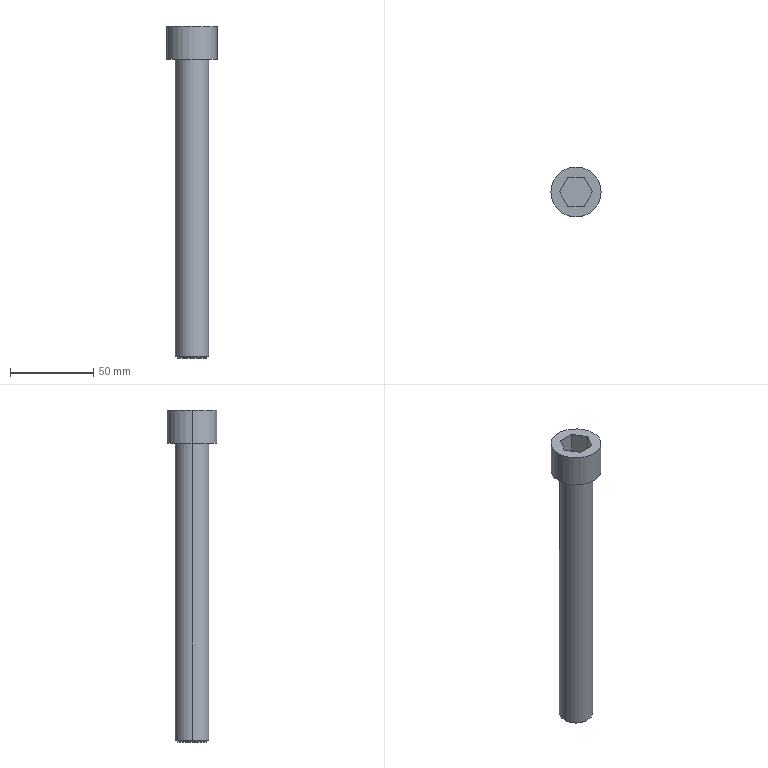Part | Creo | 1 solid | 16 faces | box 30 x 30 x 199 mm | volume 67037 mm3 | plane 10 | cylinder 4 | cone 2 | commonest cylinder face diameters 20 x2 30 x2
STEP:
#1=CARTESIAN_POINT('',(0.,0.,0.));
#2=DIRECTION('',(0.,0.,1.));
#3=DIRECTION('',(1.,0.,0.));
#4=AXIS2_PLACEMENT_3D('',#1,#2,#3);
#5=CARTESIAN_POINT('',(-295.899,-189.627,172.573));
#6=VERTEX_POINT('',#5);
#7=CARTESIAN_POINT('',(-275.899,-189.627,172.573));
#8=VERTEX_POINT('',#7);
#9=CARTESIAN_POINT('',(-285.899,-189.627,172.573));
#10=DIRECTION('',(0.,0.,-1.));
#11=DIRECTION('',(-1.,0.,0.));
#12=AXIS2_PLACEMENT_3D('',#9,#10,#11);
#13=CIRCLE('',#12,10.);
#14=EDGE_CURVE('',#6,#8,#13,.T.);
#15=ORIENTED_EDGE('',*,*,#14,.T.);
#16=CARTESIAN_POINT('',(-275.899,-189.627,350.559));
#17=VERTEX_POINT('',#16);
#18=CARTESIAN_POINT('',(-275.899,-189.627,350.559));
#19=DIRECTION('',(0.,0.,-1.));
#20=VECTOR('',#19,177.985);
#21=LINE('',#18,#20);
#22=EDGE_CURVE('',#17,#8,#21,.T.);
#23=ORIENTED_EDGE('',*,*,#22,.F.);
#24=CARTESIAN_POINT('',(-295.899,-189.627,350.559));
#25=VERTEX_POINT('',#24);
#26=CARTESIAN_POINT('',(-285.899,-189.627,350.559));
#27=DIRECTION('',(0.,0.,1.));
#28=DIRECTION('',(1.,0.,0.));
#29=AXIS2_PLACEMENT_3D('',#26,#27,#28);
#30=CIRCLE('',#29,10.);
#31=EDGE_CURVE('',#17,#25,#30,.T.);
#32=ORIENTED_EDGE('',*,*,#31,.T.);
#33=CARTESIAN_POINT('',(-295.899,-189.627,350.559));
#34=DIRECTION('',(0.,0.,-1.));
#35=VECTOR('',#34,177.985);
#36=LINE('',#33,#35);
#37=EDGE_CURVE('',#25,#6,#36,.T.);
#38=ORIENTED_EDGE('',*,*,#37,.T.);
#39=EDGE_LOOP('',(#15,#23,#32,#38));
#40=FACE_OUTER_BOUND('',#39,.F.);
#41=CARTESIAN_POINT('',(-285.899,-189.627,350.559));
#42=DIRECTION('',(0.,0.,-1.));
#43=DIRECTION('',(-1.,0.,0.));
#44=AXIS2_PLACEMENT_3D('',#41,#42,#43);
#45=CYLINDRICAL_SURFACE('',#44,10.);
#46=ADVANCED_FACE('',(#40),#45,.T.);
#47=CARTESIAN_POINT('',(-294.884,-189.627,171.559));
#48=VERTEX_POINT('',#47);
#49=CARTESIAN_POINT('',(-276.914,-189.627,171.559));
#50=VERTEX_POINT('',#49);
#51=CARTESIAN_POINT('',(-285.899,-189.627,171.559));
#52=DIRECTION('',(0.,0.,-1.));
#53=DIRECTION('',(-1.,0.,0.));
#54=AXIS2_PLACEMENT_3D('',#51,#52,#53);
#55=CIRCLE('',#54,8.985);
#56=EDGE_CURVE('',#48,#50,#55,.T.);
#57=ORIENTED_EDGE('',*,*,#56,.T.);
#58=CARTESIAN_POINT('',(-276.914,-189.627,171.559));
#59=DIRECTION('',(0.7071,0.,0.7071));
#60=VECTOR('',#59,1.435);
#61=LINE('',#58,#60);
#62=EDGE_CURVE('',#50,#8,#61,.T.);
#63=ORIENTED_EDGE('',*,*,#62,.T.);
#64=ORIENTED_EDGE('',*,*,#14,.F.);
#65=CARTESIAN_POINT('',(-294.884,-189.627,171.559));
#66=DIRECTION('',(-0.7071,0.,0.7071));
#67=VECTOR('',#66,1.435);
#68=LINE('',#65,#67);
#69=EDGE_CURVE('',#48,#6,#68,.T.);
#70=ORIENTED_EDGE('',*,*,#69,.F.);
#71=EDGE_LOOP('',(#57,#63,#64,#70));
#72=FACE_OUTER_BOUND('',#71,.F.);
#73=CARTESIAN_POINT('',(-285.899,-189.627,172.066));
#74=DIRECTION('',(0.,0.,1.));
#75=DIRECTION('',(1.,0.,0.));
#76=AXIS2_PLACEMENT_3D('',#73,#74,#75);
#77=CONICAL_SURFACE('',#76,9.493,45.);
#78=ADVANCED_FACE('',(#72),#77,.T.);
#79=CARTESIAN_POINT('',(-285.899,-189.627,171.559));
#80=DIRECTION('',(0.,0.,-1.));
#81=DIRECTION('',(1.,0.,0.));
#82=AXIS2_PLACEMENT_3D('',#79,#80,#81);
#83=CIRCLE('',#82,8.985);
#84=EDGE_CURVE('',#50,#48,#83,.T.);
#85=ORIENTED_EDGE('',*,*,#84,.F.);
#86=ORIENTED_EDGE('',*,*,#56,.F.);
#87=EDGE_LOOP('',(#85,#86));
#88=FACE_OUTER_BOUND('',#87,.F.);
#89=CARTESIAN_POINT('',(-285.899,-189.627,171.559));
#90=DIRECTION('',(0.,0.,1.));
#91=DIRECTION('',(1.,0.,0.));
#92=AXIS2_PLACEMENT_3D('',#89,#90,#91);
#93=PLANE('',#92);
#94=ADVANCED_FACE('',(#88),#93,.F.);
#95=ORIENTED_EDGE('',*,*,#84,.T.);
#96=ORIENTED_EDGE('',*,*,#69,.T.);
#97=CARTESIAN_POINT('',(-285.899,-189.627,172.573));
#98=DIRECTION('',(0.,0.,-1.));
#99=DIRECTION('',(1.,0.,0.));
#100=AXIS2_PLACEMENT_3D('',#97,#98,#99);
#101=CIRCLE('',#100,10.);
#102=EDGE_CURVE('',#8,#6,#101,.T.);
#103=ORIENTED_EDGE('',*,*,#102,.F.);
#104=ORIENTED_EDGE('',*,*,#62,.F.);
#105=EDGE_LOOP('',(#95,#96,#103,#104));
#106=FACE_OUTER_BOUND('',#105,.F.);
#107=CARTESIAN_POINT('',(-285.899,-189.627,172.066));
#108=DIRECTION('',(0.,0.,1.));
#109=DIRECTION('',(1.,0.,0.));
#110=AXIS2_PLACEMENT_3D('',#107,#108,#109);
#111=CONICAL_SURFACE('',#110,9.493,45.);
#112=ADVANCED_FACE('',(#106),#111,.T.);
#113=ORIENTED_EDGE('',*,*,#102,.T.);
#114=ORIENTED_EDGE('',*,*,#37,.F.);
#115=CARTESIAN_POINT('',(-285.899,-189.627,350.559));
#116=DIRECTION('',(0.,0.,1.));
#117=DIRECTION('',(-1.,0.,0.));
#118=AXIS2_PLACEMENT_3D('',#115,#116,#117);
#119=CIRCLE('',#118,10.);
#120=EDGE_CURVE('',#25,#17,#119,.T.);
#121=ORIENTED_EDGE('',*,*,#120,.T.);
#122=ORIENTED_EDGE('',*,*,#22,.T.);
#123=EDGE_LOOP('',(#113,#114,#121,#122));
#124=FACE_OUTER_BOUND('',#123,.F.);
#125=CARTESIAN_POINT('',(-285.899,-189.627,350.559));
#126=DIRECTION('',(0.,0.,-1.));
#127=DIRECTION('',(-1.,0.,0.));
#128=AXIS2_PLACEMENT_3D('',#125,#126,#127);
#129=CYLINDRICAL_SURFACE('',#128,10.);
#130=ADVANCED_FACE('',(#124),#129,.T.);
#131=CARTESIAN_POINT('',(-270.899,-189.627,350.559));
#132=VERTEX_POINT('',#131);
#133=CARTESIAN_POINT('',(-300.899,-189.627,350.559));
#134=VERTEX_POINT('',#133);
#135=CARTESIAN_POINT('',(-285.899,-189.627,350.559));
#136=DIRECTION('',(0.,0.,-1.));
#137=DIRECTION('',(1.,0.,0.));
#138=AXIS2_PLACEMENT_3D('',#135,#136,#137);
#139=CIRCLE('',#138,15.);
#140=EDGE_CURVE('',#132,#134,#139,.T.);
#141=ORIENTED_EDGE('',*,*,#140,.F.);
#142=CARTESIAN_POINT('',(-285.899,-189.627,350.559));
#143=DIRECTION('',(0.,0.,-1.));
#144=DIRECTION('',(-1.,0.,0.));
#145=AXIS2_PLACEMENT_3D('',#142,#143,#144);
#146=CIRCLE('',#145,15.);
#147=EDGE_CURVE('',#134,#132,#146,.T.);
#148=ORIENTED_EDGE('',*,*,#147,.F.);
#149=EDGE_LOOP('',(#141,#148));
#150=FACE_OUTER_BOUND('',#149,.F.);
#151=ORIENTED_EDGE('',*,*,#31,.F.);
#152=ORIENTED_EDGE('',*,*,#120,.F.);
#153=EDGE_LOOP('',(#151,#152));
#154=FACE_BOUND('',#153,.F.);
#155=CARTESIAN_POINT('',(-285.899,-189.627,350.559));
#156=DIRECTION('',(0.,0.,-1.));
#157=DIRECTION('',(-1.,0.,0.));
#158=AXIS2_PLACEMENT_3D('',#155,#156,#157);
#159=PLANE('',#158);
#160=ADVANCED_FACE('',(#150,#154),#159,.T.);
#161=CARTESIAN_POINT('',(-300.899,-189.627,370.559));
#162=VERTEX_POINT('',#161);
#163=CARTESIAN_POINT('',(-270.899,-189.627,370.559));
#164=VERTEX_POINT('',#163);
#165=CARTESIAN_POINT('',(-285.899,-189.627,370.559));
#166=DIRECTION('',(0.,0.,1.));
#167=DIRECTION('',(-1.,0.,0.));
#168=AXIS2_PLACEMENT_3D('',#165,#166,#167);
#169=CIRCLE('',#168,15.);
#170=EDGE_CURVE('',#162,#164,#169,.T.);
#171=ORIENTED_EDGE('',*,*,#170,.T.);
#172=CARTESIAN_POINT('',(-270.899,-189.627,350.559));
#173=DIRECTION('',(0.,0.,1.));
#174=VECTOR('',#173,20.);
#175=LINE('',#172,#174);
#176=EDGE_CURVE('',#132,#164,#175,.T.);
#177=ORIENTED_EDGE('',*,*,#176,.F.);
#178=ORIENTED_EDGE('',*,*,#140,.T.);
#179=CARTESIAN_POINT('',(-300.899,-189.627,350.559));
#180=DIRECTION('',(0.,0.,1.));
#181=VECTOR('',#180,20.);
#182=LINE('',#179,#181);
#183=EDGE_CURVE('',#134,#162,#182,.T.);
#184=ORIENTED_EDGE('',*,*,#183,.T.);
#185=EDGE_LOOP('',(#171,#177,#178,#184));
#186=FACE_OUTER_BOUND('',#185,.F.);
#187=CARTESIAN_POINT('',(-285.899,-189.627,350.559));
#188=DIRECTION('',(0.,0.,1.));
#189=DIRECTION('',(1.,0.,0.));
#190=AXIS2_PLACEMENT_3D('',#187,#188,#189);
#191=CYLINDRICAL_SURFACE('',#190,15.);
#192=ADVANCED_FACE('',(#186),#191,.T.);
#193=CARTESIAN_POINT('',(-285.899,-189.627,370.559));
#194=DIRECTION('',(0.,0.,1.));
#195=DIRECTION('',(1.,0.,0.));
#196=AXIS2_PLACEMENT_3D('',#193,#194,#195);
#197=CIRCLE('',#196,15.);
#198=EDGE_CURVE('',#164,#162,#197,.T.);
#199=ORIENTED_EDGE('',*,*,#198,.F.);
#200=ORIENTED_EDGE('',*,*,#170,.F.);
#201=EDGE_LOOP('',(#199,#200));
#202=FACE_OUTER_BOUND('',#201,.F.);
#203=CARTESIAN_POINT('',(-280.992,-198.127,370.559));
#204=VERTEX_POINT('',#203);
#205=CARTESIAN_POINT('',(-290.807,-198.127,370.559));
#206=VERTEX_POINT('',#205);
#207=CARTESIAN_POINT('',(-280.992,-198.127,370.559));
#208=DIRECTION('',(-1.,0.,0.));
#209=VECTOR('',#208,9.815);
#210=LINE('',#207,#209);
#211=EDGE_CURVE('',#204,#206,#210,.T.);
#212=ORIENTED_EDGE('',*,*,#211,.F.);
#213=CARTESIAN_POINT('',(-276.084,-189.627,370.559));
#214=VERTEX_POINT('',#213);
#215=CARTESIAN_POINT('',(-276.084,-189.627,370.559));
#216=DIRECTION('',(-0.5,-0.866,0.));
#217=VECTOR('',#216,9.815);
#218=LINE('',#215,#217);
#219=EDGE_CURVE('',#214,#204,#218,.T.);
#220=ORIENTED_EDGE('',*,*,#219,.F.);
#221=CARTESIAN_POINT('',(-280.992,-181.127,370.559));
#222=VERTEX_POINT('',#221);
#223=CARTESIAN_POINT('',(-280.992,-181.127,370.559));
#224=DIRECTION('',(0.5,-0.866,0.));
#225=VECTOR('',#224,9.815);
#226=LINE('',#223,#225);
#227=EDGE_CURVE('',#222,#214,#226,.T.);
#228=ORIENTED_EDGE('',*,*,#227,.F.);
#229=CARTESIAN_POINT('',(-290.807,-181.127,370.559));
#230=VERTEX_POINT('',#229);
#231=CARTESIAN_POINT('',(-290.807,-181.127,370.559));
#232=DIRECTION('',(1.,0.,0.));
#233=VECTOR('',#232,9.815);
#234=LINE('',#231,#233);
#235=EDGE_CURVE('',#230,#222,#234,.T.);
#236=ORIENTED_EDGE('',*,*,#235,.F.);
#237=CARTESIAN_POINT('',(-295.714,-189.627,370.559));
#238=VERTEX_POINT('',#237);
#239=CARTESIAN_POINT('',(-295.714,-189.627,370.559));
#240=DIRECTION('',(0.5,0.866,0.));
#241=VECTOR('',#240,9.815);
#242=LINE('',#239,#241);
#243=EDGE_CURVE('',#238,#230,#242,.T.);
#244=ORIENTED_EDGE('',*,*,#243,.F.);
#245=CARTESIAN_POINT('',(-290.807,-198.127,370.559));
#246=DIRECTION('',(-0.5,0.866,0.));
#247=VECTOR('',#246,9.815);
#248=LINE('',#245,#247);
#249=EDGE_CURVE('',#206,#238,#248,.T.);
#250=ORIENTED_EDGE('',*,*,#249,.F.);
#251=EDGE_LOOP('',(#212,#220,#228,#236,#244,#250));
#252=FACE_BOUND('',#251,.F.);
#253=CARTESIAN_POINT('',(-285.899,-189.627,370.559));
#254=DIRECTION('',(0.,0.,1.));
#255=DIRECTION('',(1.,0.,0.));
#256=AXIS2_PLACEMENT_3D('',#253,#254,#255);
#257=PLANE('',#256);
#258=ADVANCED_FACE('',(#202,#252),#257,.T.);
#259=ORIENTED_EDGE('',*,*,#211,.T.);
#260=CARTESIAN_POINT('',(-290.807,-198.127,357.359));
#261=VERTEX_POINT('',#260);
#262=CARTESIAN_POINT('',(-290.807,-198.127,370.559));
#263=DIRECTION('',(0.,0.,-1.));
#264=VECTOR('',#263,13.2);
#265=LINE('',#262,#264);
#266=EDGE_CURVE('',#206,#261,#265,.T.);
#267=ORIENTED_EDGE('',*,*,#266,.T.);
#268=CARTESIAN_POINT('',(-280.992,-198.127,357.359));
#269=VERTEX_POINT('',#268);
#270=CARTESIAN_POINT('',(-280.992,-198.127,357.359));
#271=DIRECTION('',(-1.,0.,0.));
#272=VECTOR('',#271,9.815);
#273=LINE('',#270,#272);
#274=EDGE_CURVE('',#269,#261,#273,.T.);
#275=ORIENTED_EDGE('',*,*,#274,.F.);
#276=CARTESIAN_POINT('',(-280.992,-198.127,370.559));
#277=DIRECTION('',(0.,0.,-1.));
#278=VECTOR('',#277,13.2);
#279=LINE('',#276,#278);
#280=EDGE_CURVE('',#204,#269,#279,.T.);
#281=ORIENTED_EDGE('',*,*,#280,.F.);
#282=EDGE_LOOP('',(#259,#267,#275,#281));
#283=FACE_OUTER_BOUND('',#282,.F.);
#284=CARTESIAN_POINT('',(-290.807,-198.127,357.359));
#285=DIRECTION('',(0.,-1.,0.));
#286=DIRECTION('',(0.,0.,-1.));
#287=AXIS2_PLACEMENT_3D('',#284,#285,#286);
#288=PLANE('',#287);
#289=ADVANCED_FACE('',(#283),#288,.F.);
#290=ORIENTED_EDGE('',*,*,#249,.T.);
#291=CARTESIAN_POINT('',(-295.714,-189.627,357.359));
#292=VERTEX_POINT('',#291);
#293=CARTESIAN_POINT('',(-295.714,-189.627,370.559));
#294=DIRECTION('',(0.,0.,-1.));
#295=VECTOR('',#294,13.2);
#296=LINE('',#293,#295);
#297=EDGE_CURVE('',#238,#292,#296,.T.);
#298=ORIENTED_EDGE('',*,*,#297,.T.);
#299=CARTESIAN_POINT('',(-295.714,-189.627,357.359));
#300=DIRECTION('',(0.5,-0.866,0.));
#301=VECTOR('',#300,9.815);
#302=LINE('',#299,#301);
#303=EDGE_CURVE('',#292,#261,#302,.T.);
#304=ORIENTED_EDGE('',*,*,#303,.T.);
#305=ORIENTED_EDGE('',*,*,#266,.F.);
#306=EDGE_LOOP('',(#290,#298,#304,#305));
#307=FACE_OUTER_BOUND('',#306,.F.);
#308=CARTESIAN_POINT('',(-295.714,-189.627,357.359));
#309=DIRECTION('',(-0.866,-0.5,0.));
#310=DIRECTION('',(0.5,-0.866,0.));
#311=AXIS2_PLACEMENT_3D('',#308,#309,#310);
#312=PLANE('',#311);
#313=ADVANCED_FACE('',(#307),#312,.F.);
#314=ORIENTED_EDGE('',*,*,#243,.T.);
#315=CARTESIAN_POINT('',(-290.807,-181.127,357.359));
#316=VERTEX_POINT('',#315);
#317=CARTESIAN_POINT('',(-290.807,-181.127,370.559));
#318=DIRECTION('',(0.,0.,-1.));
#319=VECTOR('',#318,13.2);
#320=LINE('',#317,#319);
#321=EDGE_CURVE('',#230,#316,#320,.T.);
#322=ORIENTED_EDGE('',*,*,#321,.T.);
#323=CARTESIAN_POINT('',(-290.807,-181.127,357.359));
#324=DIRECTION('',(-0.5,-0.866,0.));
#325=VECTOR('',#324,9.815);
#326=LINE('',#323,#325);
#327=EDGE_CURVE('',#316,#292,#326,.T.);
#328=ORIENTED_EDGE('',*,*,#327,.T.);
#329=ORIENTED_EDGE('',*,*,#297,.F.);
#330=EDGE_LOOP('',(#314,#322,#328,#329));
#331=FACE_OUTER_BOUND('',#330,.F.);
#332=CARTESIAN_POINT('',(-290.807,-181.127,357.359));
#333=DIRECTION('',(-0.866,0.5,0.));
#334=DIRECTION('',(-0.5,-0.866,0.));
#335=AXIS2_PLACEMENT_3D('',#332,#333,#334);
#336=PLANE('',#335);
#337=ADVANCED_FACE('',(#331),#336,.F.);
#338=ORIENTED_EDGE('',*,*,#235,.T.);
#339=CARTESIAN_POINT('',(-280.992,-181.127,357.359));
#340=VERTEX_POINT('',#339);
#341=CARTESIAN_POINT('',(-280.992,-181.127,370.559));
#342=DIRECTION('',(0.,0.,-1.));
#343=VECTOR('',#342,13.2);
#344=LINE('',#341,#343);
#345=EDGE_CURVE('',#222,#340,#344,.T.);
#346=ORIENTED_EDGE('',*,*,#345,.T.);
#347=CARTESIAN_POINT('',(-290.807,-181.127,357.359));
#348=DIRECTION('',(1.,0.,0.));
#349=VECTOR('',#348,9.815);
#350=LINE('',#347,#349);
#351=EDGE_CURVE('',#316,#340,#350,.T.);
#352=ORIENTED_EDGE('',*,*,#351,.F.);
#353=ORIENTED_EDGE('',*,*,#321,.F.);
#354=EDGE_LOOP('',(#338,#346,#352,#353));
#355=FACE_OUTER_BOUND('',#354,.F.);
#356=CARTESIAN_POINT('',(-280.992,-181.127,357.359));
#357=DIRECTION('',(0.,1.,0.));
#358=DIRECTION('',(0.,0.,1.));
#359=AXIS2_PLACEMENT_3D('',#356,#357,#358);
#360=PLANE('',#359);
#361=ADVANCED_FACE('',(#355),#360,.F.);
#362=ORIENTED_EDGE('',*,*,#227,.T.);
#363=CARTESIAN_POINT('',(-276.084,-189.627,357.359));
#364=VERTEX_POINT('',#363);
#365=CARTESIAN_POINT('',(-276.084,-189.627,370.559));
#366=DIRECTION('',(0.,0.,-1.));
#367=VECTOR('',#366,13.2);
#368=LINE('',#365,#367);
#369=EDGE_CURVE('',#214,#364,#368,.T.);
#370=ORIENTED_EDGE('',*,*,#369,.T.);
#371=CARTESIAN_POINT('',(-276.084,-189.627,357.359));
#372=DIRECTION('',(-0.5,0.866,0.));
#373=VECTOR('',#372,9.815);
#374=LINE('',#371,#373);
#375=EDGE_CURVE('',#364,#340,#374,.T.);
#376=ORIENTED_EDGE('',*,*,#375,.T.);
#377=ORIENTED_EDGE('',*,*,#345,.F.);
#378=EDGE_LOOP('',(#362,#370,#376,#377));
#379=FACE_OUTER_BOUND('',#378,.F.);
#380=CARTESIAN_POINT('',(-276.084,-189.627,357.359));
#381=DIRECTION('',(0.866,0.5,0.));
#382=DIRECTION('',(-0.5,0.866,0.));
#383=AXIS2_PLACEMENT_3D('',#380,#381,#382);
#384=PLANE('',#383);
#385=ADVANCED_FACE('',(#379),#384,.F.);
#386=ORIENTED_EDGE('',*,*,#219,.T.);
#387=ORIENTED_EDGE('',*,*,#280,.T.);
#388=CARTESIAN_POINT('',(-280.992,-198.127,357.359));
#389=DIRECTION('',(0.5,0.866,0.));
#390=VECTOR('',#389,9.815);
#391=LINE('',#388,#390);
#392=EDGE_CURVE('',#269,#364,#391,.T.);
#393=ORIENTED_EDGE('',*,*,#392,.T.);
#394=ORIENTED_EDGE('',*,*,#369,.F.);
#395=EDGE_LOOP('',(#386,#387,#393,#394));
#396=FACE_OUTER_BOUND('',#395,.F.);
#397=CARTESIAN_POINT('',(-280.992,-198.127,357.359));
#398=DIRECTION('',(0.866,-0.5,0.));
#399=DIRECTION('',(0.5,0.866,0.));
#400=AXIS2_PLACEMENT_3D('',#397,#398,#399);
#401=PLANE('',#400);
#402=ADVANCED_FACE('',(#396),#401,.F.);
#403=ORIENTED_EDGE('',*,*,#274,.T.);
#404=ORIENTED_EDGE('',*,*,#303,.F.);
#405=ORIENTED_EDGE('',*,*,#327,.F.);
#406=ORIENTED_EDGE('',*,*,#351,.T.);
#407=ORIENTED_EDGE('',*,*,#375,.F.);
#408=ORIENTED_EDGE('',*,*,#392,.F.);
#409=EDGE_LOOP('',(#403,#404,#405,#406,#407,#408));
#410=FACE_OUTER_BOUND('',#409,.F.);
#411=CARTESIAN_POINT('',(-280.992,-198.127,357.359));
#412=DIRECTION('',(0.,0.,1.));
#413=DIRECTION('',(1.,0.,0.));
#414=AXIS2_PLACEMENT_3D('',#411,#412,#413);
#415=PLANE('',#414);
#416=ADVANCED_FACE('',(#410),#415,.T.);
#417=ORIENTED_EDGE('',*,*,#198,.T.);
#418=ORIENTED_EDGE('',*,*,#183,.F.);
#419=ORIENTED_EDGE('',*,*,#147,.T.);
#420=ORIENTED_EDGE('',*,*,#176,.T.);
#421=EDGE_LOOP('',(#417,#418,#419,#420));
#422=FACE_OUTER_BOUND('',#421,.F.);
#423=CARTESIAN_POINT('',(-285.899,-189.627,350.559));
#424=DIRECTION('',(0.,0.,1.));
#425=DIRECTION('',(1.,0.,0.));
#426=AXIS2_PLACEMENT_3D('',#423,#424,#425);
#427=CYLINDRICAL_SURFACE('',#426,15.);
#428=ADVANCED_FACE('',(#422),#427,.T.);
#429=CLOSED_SHELL('',(#46,#78,#94,#112,#130,#160,#192,#258,#289,#313,#337,#361,#385,#402,#416,#428));
#430=MANIFOLD_SOLID_BREP('',#429);
#431=(LENGTH_UNIT()NAMED_UNIT(*)SI_UNIT(.MILLI.,.METRE.));
#432=UNCERTAINTY_MEASURE_WITH_UNIT(LENGTH_MEASURE(0.02035),#431,'','');
#433=(NAMED_UNIT(*)PLANE_ANGLE_UNIT()SI_UNIT($,.RADIAN.));
#434=PLANE_ANGLE_MEASURE_WITH_UNIT(PLANE_ANGLE_MEASURE(0.01745),#433);
#435=(CONVERSION_BASED_UNIT('DEGREE',#434)NAMED_UNIT(*)PLANE_ANGLE_UNIT());
#436=(NAMED_UNIT(*)SI_UNIT($,.STERADIAN.)SOLID_ANGLE_UNIT());
#437=(GEOMETRIC_REPRESENTATION_CONTEXT(3)GLOBAL_UNCERTAINTY_ASSIGNED_CONTEXT((#432))GLOBAL_UNIT_ASSIGNED_CONTEXT((#431,#435,#436))REPRESENTATION_CONTEXT('',''));
#438=ADVANCED_BREP_SHAPE_REPRESENTATION('',(#4,#430),#437);